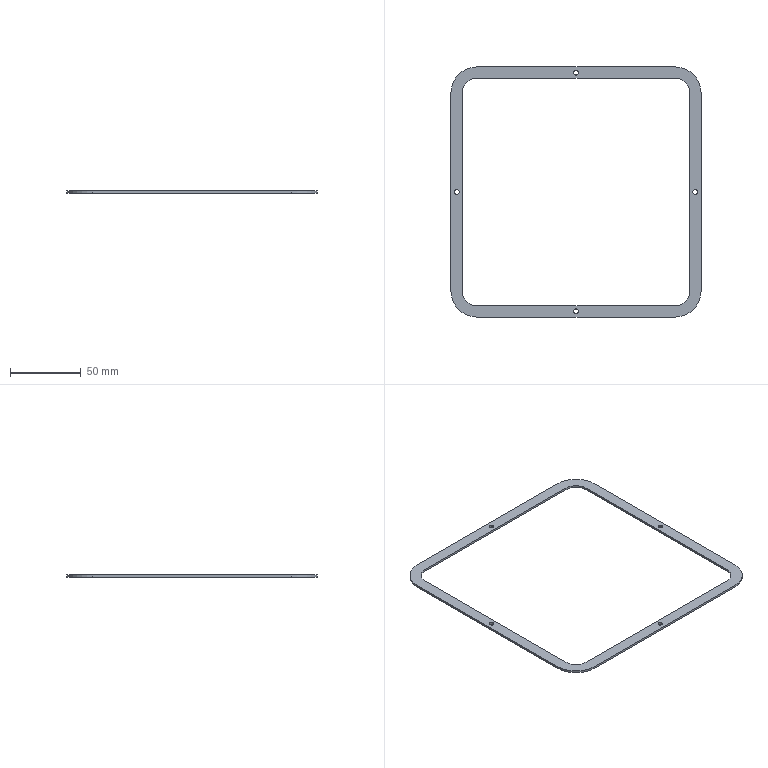Part | NX | features BREP 1 | 1 solid | 26 faces | box 176.2 x 176.2 x 1.5 mm | volume 7641 mm3 | cylinder 16 | plane 10 | commonest cylinder face diameters 3.2 x8 20.4 x4 36.2 x4
STEP:
#1=CARTESIAN_POINT('',(99.822,29.098,1.5));
#2=VERTEX_POINT('',#1);
#3=CARTESIAN_POINT('',(103.022,29.098,1.5));
#4=VERTEX_POINT('',#3);
#5=CARTESIAN_POINT('',(101.422,29.098,1.5));
#6=DIRECTION('',(0.,0.,1.));
#7=DIRECTION('',(1.,0.,0.));
#8=AXIS2_PLACEMENT_3D('',#5,#6,#7);
#9=CIRCLE('',#8,1.6);
#10=EDGE_CURVE('',#2,#4,#9,.T.);
#11=ORIENTED_EDGE('',*,*,#10,.T.);
#12=CARTESIAN_POINT('',(103.022,29.098,0.));
#13=VERTEX_POINT('',#12);
#14=CARTESIAN_POINT('',(103.022,29.098,1.5));
#15=DIRECTION('',(0.,0.,-1.));
#16=VECTOR('',#15,1000.);
#17=LINE('',#14,#16);
#18=EDGE_CURVE('',#13,#4,#17,.F.);
#19=ORIENTED_EDGE('',*,*,#18,.F.);
#20=CARTESIAN_POINT('',(99.822,29.098,0.));
#21=VERTEX_POINT('',#20);
#22=CARTESIAN_POINT('',(101.422,29.098,0.));
#23=DIRECTION('',(0.,0.,1.));
#24=DIRECTION('',(1.,0.,0.));
#25=AXIS2_PLACEMENT_3D('',#22,#23,#24);
#26=CIRCLE('',#25,1.6);
#27=EDGE_CURVE('',#21,#13,#26,.T.);
#28=ORIENTED_EDGE('',*,*,#27,.F.);
#29=CARTESIAN_POINT('',(99.822,29.098,1.5));
#30=DIRECTION('',(0.,0.,-1.));
#31=VECTOR('',#30,1000.);
#32=LINE('',#29,#31);
#33=EDGE_CURVE('',#21,#2,#32,.F.);
#34=ORIENTED_EDGE('',*,*,#33,.T.);
#35=EDGE_LOOP('',(#11,#19,#28,#34));
#36=FACE_BOUND('',#35,.T.);
#37=CARTESIAN_POINT('',(101.422,29.098,1.5));
#38=DIRECTION('',(0.,0.,-1.));
#39=DIRECTION('',(1.,0.,0.));
#40=AXIS2_PLACEMENT_3D('',#37,#38,#39);
#41=CYLINDRICAL_SURFACE('',#40,1.6);
#42=ADVANCED_FACE('',(#36),#41,.F.);
#43=CARTESIAN_POINT('',(15.822,-54.902,1.5));
#44=VERTEX_POINT('',#43);
#45=CARTESIAN_POINT('',(19.022,-54.902,1.5));
#46=VERTEX_POINT('',#45);
#47=CARTESIAN_POINT('',(17.422,-54.902,1.5));
#48=DIRECTION('',(0.,0.,1.));
#49=DIRECTION('',(1.,0.,0.));
#50=AXIS2_PLACEMENT_3D('',#47,#48,#49);
#51=CIRCLE('',#50,1.6);
#52=EDGE_CURVE('',#44,#46,#51,.T.);
#53=ORIENTED_EDGE('',*,*,#52,.T.);
#54=CARTESIAN_POINT('',(19.022,-54.902,0.));
#55=VERTEX_POINT('',#54);
#56=CARTESIAN_POINT('',(19.022,-54.902,1.5));
#57=DIRECTION('',(0.,0.,-1.));
#58=VECTOR('',#57,1000.);
#59=LINE('',#56,#58);
#60=EDGE_CURVE('',#55,#46,#59,.F.);
#61=ORIENTED_EDGE('',*,*,#60,.F.);
#62=CARTESIAN_POINT('',(15.822,-54.902,0.));
#63=VERTEX_POINT('',#62);
#64=CARTESIAN_POINT('',(17.422,-54.902,0.));
#65=DIRECTION('',(0.,0.,1.));
#66=DIRECTION('',(1.,0.,0.));
#67=AXIS2_PLACEMENT_3D('',#64,#65,#66);
#68=CIRCLE('',#67,1.6);
#69=EDGE_CURVE('',#63,#55,#68,.T.);
#70=ORIENTED_EDGE('',*,*,#69,.F.);
#71=CARTESIAN_POINT('',(15.822,-54.902,1.5));
#72=DIRECTION('',(0.,0.,-1.));
#73=VECTOR('',#72,1000.);
#74=LINE('',#71,#73);
#75=EDGE_CURVE('',#63,#44,#74,.F.);
#76=ORIENTED_EDGE('',*,*,#75,.T.);
#77=EDGE_LOOP('',(#53,#61,#70,#76));
#78=FACE_BOUND('',#77,.T.);
#79=CARTESIAN_POINT('',(17.422,-54.902,1.5));
#80=DIRECTION('',(0.,0.,-1.));
#81=DIRECTION('',(1.,0.,0.));
#82=AXIS2_PLACEMENT_3D('',#79,#80,#81);
#83=CYLINDRICAL_SURFACE('',#82,1.6);
#84=ADVANCED_FACE('',(#78),#83,.F.);
#85=CARTESIAN_POINT('',(-68.178,29.098,1.5));
#86=VERTEX_POINT('',#85);
#87=CARTESIAN_POINT('',(-64.978,29.098,1.5));
#88=VERTEX_POINT('',#87);
#89=CARTESIAN_POINT('',(-66.578,29.098,1.5));
#90=DIRECTION('',(0.,0.,1.));
#91=DIRECTION('',(1.,0.,0.));
#92=AXIS2_PLACEMENT_3D('',#89,#90,#91);
#93=CIRCLE('',#92,1.6);
#94=EDGE_CURVE('',#86,#88,#93,.T.);
#95=ORIENTED_EDGE('',*,*,#94,.T.);
#96=CARTESIAN_POINT('',(-64.978,29.098,0.));
#97=VERTEX_POINT('',#96);
#98=CARTESIAN_POINT('',(-64.978,29.098,1.5));
#99=DIRECTION('',(0.,0.,-1.));
#100=VECTOR('',#99,1000.);
#101=LINE('',#98,#100);
#102=EDGE_CURVE('',#97,#88,#101,.F.);
#103=ORIENTED_EDGE('',*,*,#102,.F.);
#104=CARTESIAN_POINT('',(-68.178,29.098,0.));
#105=VERTEX_POINT('',#104);
#106=CARTESIAN_POINT('',(-66.578,29.098,0.));
#107=DIRECTION('',(0.,0.,1.));
#108=DIRECTION('',(1.,0.,0.));
#109=AXIS2_PLACEMENT_3D('',#106,#107,#108);
#110=CIRCLE('',#109,1.6);
#111=EDGE_CURVE('',#105,#97,#110,.T.);
#112=ORIENTED_EDGE('',*,*,#111,.F.);
#113=CARTESIAN_POINT('',(-68.178,29.098,1.5));
#114=DIRECTION('',(0.,0.,-1.));
#115=VECTOR('',#114,1000.);
#116=LINE('',#113,#115);
#117=EDGE_CURVE('',#105,#86,#116,.F.);
#118=ORIENTED_EDGE('',*,*,#117,.T.);
#119=EDGE_LOOP('',(#95,#103,#112,#118));
#120=FACE_BOUND('',#119,.T.);
#121=CARTESIAN_POINT('',(-66.578,29.098,1.5));
#122=DIRECTION('',(0.,0.,-1.));
#123=DIRECTION('',(1.,0.,0.));
#124=AXIS2_PLACEMENT_3D('',#121,#122,#123);
#125=CYLINDRICAL_SURFACE('',#124,1.6);
#126=ADVANCED_FACE('',(#120),#125,.F.);
#127=CARTESIAN_POINT('',(15.822,113.098,1.5));
#128=VERTEX_POINT('',#127);
#129=CARTESIAN_POINT('',(19.022,113.098,1.5));
#130=VERTEX_POINT('',#129);
#131=CARTESIAN_POINT('',(17.422,113.098,1.5));
#132=DIRECTION('',(0.,0.,1.));
#133=DIRECTION('',(1.,0.,0.));
#134=AXIS2_PLACEMENT_3D('',#131,#132,#133);
#135=CIRCLE('',#134,1.6);
#136=EDGE_CURVE('',#128,#130,#135,.T.);
#137=ORIENTED_EDGE('',*,*,#136,.T.);
#138=CARTESIAN_POINT('',(19.022,113.098,0.));
#139=VERTEX_POINT('',#138);
#140=CARTESIAN_POINT('',(19.022,113.098,1.5));
#141=DIRECTION('',(0.,0.,-1.));
#142=VECTOR('',#141,1000.);
#143=LINE('',#140,#142);
#144=EDGE_CURVE('',#139,#130,#143,.F.);
#145=ORIENTED_EDGE('',*,*,#144,.F.);
#146=CARTESIAN_POINT('',(15.822,113.098,0.));
#147=VERTEX_POINT('',#146);
#148=CARTESIAN_POINT('',(17.422,113.098,0.));
#149=DIRECTION('',(0.,0.,1.));
#150=DIRECTION('',(1.,0.,0.));
#151=AXIS2_PLACEMENT_3D('',#148,#149,#150);
#152=CIRCLE('',#151,1.6);
#153=EDGE_CURVE('',#147,#139,#152,.T.);
#154=ORIENTED_EDGE('',*,*,#153,.F.);
#155=CARTESIAN_POINT('',(15.822,113.098,1.5));
#156=DIRECTION('',(0.,0.,-1.));
#157=VECTOR('',#156,1000.);
#158=LINE('',#155,#157);
#159=EDGE_CURVE('',#147,#128,#158,.F.);
#160=ORIENTED_EDGE('',*,*,#159,.T.);
#161=EDGE_LOOP('',(#137,#145,#154,#160));
#162=FACE_BOUND('',#161,.T.);
#163=CARTESIAN_POINT('',(17.422,113.098,1.5));
#164=DIRECTION('',(0.,0.,-1.));
#165=DIRECTION('',(1.,0.,0.));
#166=AXIS2_PLACEMENT_3D('',#163,#164,#165);
#167=CYLINDRICAL_SURFACE('',#166,1.6);
#168=ADVANCED_FACE('',(#162),#167,.F.);
#169=CARTESIAN_POINT('',(-70.678,-40.902,1.5));
#170=VERTEX_POINT('',#169);
#171=CARTESIAN_POINT('',(-52.578,-59.002,1.5));
#172=VERTEX_POINT('',#171);
#173=CARTESIAN_POINT('',(-52.578,-40.902,1.5));
#174=DIRECTION('',(0.,0.,1.));
#175=DIRECTION('',(1.,0.,0.));
#176=AXIS2_PLACEMENT_3D('',#173,#174,#175);
#177=CIRCLE('',#176,18.1);
#178=EDGE_CURVE('',#170,#172,#177,.T.);
#179=ORIENTED_EDGE('',*,*,#178,.T.);
#180=CARTESIAN_POINT('',(87.422,-59.002,1.5));
#181=VERTEX_POINT('',#180);
#182=CARTESIAN_POINT('',(-52.578,-59.002,1.5));
#183=DIRECTION('',(1.,0.,0.));
#184=VECTOR('',#183,1000.);
#185=LINE('',#182,#184);
#186=EDGE_CURVE('',#172,#181,#185,.T.);
#187=ORIENTED_EDGE('',*,*,#186,.T.);
#188=CARTESIAN_POINT('',(105.522,-40.902,1.5));
#189=VERTEX_POINT('',#188);
#190=CARTESIAN_POINT('',(87.422,-40.902,1.5));
#191=DIRECTION('',(0.,0.,1.));
#192=DIRECTION('',(1.,0.,0.));
#193=AXIS2_PLACEMENT_3D('',#190,#191,#192);
#194=CIRCLE('',#193,18.1);
#195=EDGE_CURVE('',#181,#189,#194,.T.);
#196=ORIENTED_EDGE('',*,*,#195,.T.);
#197=CARTESIAN_POINT('',(105.522,99.098,1.5));
#198=VERTEX_POINT('',#197);
#199=CARTESIAN_POINT('',(105.522,-40.902,1.5));
#200=DIRECTION('',(0.,1.,0.));
#201=VECTOR('',#200,1000.);
#202=LINE('',#199,#201);
#203=EDGE_CURVE('',#189,#198,#202,.T.);
#204=ORIENTED_EDGE('',*,*,#203,.T.);
#205=CARTESIAN_POINT('',(87.422,117.198,1.5));
#206=VERTEX_POINT('',#205);
#207=CARTESIAN_POINT('',(87.422,99.098,1.5));
#208=DIRECTION('',(0.,0.,1.));
#209=DIRECTION('',(1.,0.,0.));
#210=AXIS2_PLACEMENT_3D('',#207,#208,#209);
#211=CIRCLE('',#210,18.1);
#212=EDGE_CURVE('',#198,#206,#211,.T.);
#213=ORIENTED_EDGE('',*,*,#212,.T.);
#214=CARTESIAN_POINT('',(-52.578,117.198,1.5));
#215=VERTEX_POINT('',#214);
#216=CARTESIAN_POINT('',(87.422,117.198,1.5));
#217=DIRECTION('',(-1.,0.,0.));
#218=VECTOR('',#217,1000.);
#219=LINE('',#216,#218);
#220=EDGE_CURVE('',#206,#215,#219,.T.);
#221=ORIENTED_EDGE('',*,*,#220,.T.);
#222=CARTESIAN_POINT('',(-70.678,99.098,1.5));
#223=VERTEX_POINT('',#222);
#224=CARTESIAN_POINT('',(-52.578,99.098,1.5));
#225=DIRECTION('',(0.,0.,1.));
#226=DIRECTION('',(1.,0.,0.));
#227=AXIS2_PLACEMENT_3D('',#224,#225,#226);
#228=CIRCLE('',#227,18.1);
#229=EDGE_CURVE('',#215,#223,#228,.T.);
#230=ORIENTED_EDGE('',*,*,#229,.T.);
#231=CARTESIAN_POINT('',(-70.678,99.098,1.5));
#232=DIRECTION('',(0.,-1.,0.));
#233=VECTOR('',#232,1000.);
#234=LINE('',#231,#233);
#235=EDGE_CURVE('',#223,#170,#234,.T.);
#236=ORIENTED_EDGE('',*,*,#235,.T.);
#237=EDGE_LOOP('',(#179,#187,#196,#204,#213,#221,#230,#236));
#238=FACE_BOUND('',#237,.T.);
#239=ORIENTED_EDGE('',*,*,#52,.F.);
#240=CARTESIAN_POINT('',(17.422,-54.902,1.5));
#241=DIRECTION('',(0.,0.,1.));
#242=DIRECTION('',(1.,0.,0.));
#243=AXIS2_PLACEMENT_3D('',#240,#241,#242);
#244=CIRCLE('',#243,1.6);
#245=EDGE_CURVE('',#46,#44,#244,.T.);
#246=ORIENTED_EDGE('',*,*,#245,.F.);
#247=EDGE_LOOP('',(#239,#246));
#248=FACE_BOUND('',#247,.T.);
#249=ORIENTED_EDGE('',*,*,#136,.F.);
#250=CARTESIAN_POINT('',(17.422,113.098,1.5));
#251=DIRECTION('',(0.,0.,1.));
#252=DIRECTION('',(1.,0.,0.));
#253=AXIS2_PLACEMENT_3D('',#250,#251,#252);
#254=CIRCLE('',#253,1.6);
#255=EDGE_CURVE('',#130,#128,#254,.T.);
#256=ORIENTED_EDGE('',*,*,#255,.F.);
#257=EDGE_LOOP('',(#249,#256));
#258=FACE_BOUND('',#257,.T.);
#259=CARTESIAN_POINT('',(-52.578,-51.102,1.5));
#260=VERTEX_POINT('',#259);
#261=CARTESIAN_POINT('',(87.422,-51.102,1.5));
#262=VERTEX_POINT('',#261);
#263=CARTESIAN_POINT('',(-52.578,-51.102,1.5));
#264=DIRECTION('',(1.,0.,0.));
#265=VECTOR('',#264,1000.);
#266=LINE('',#263,#265);
#267=EDGE_CURVE('',#260,#262,#266,.T.);
#268=ORIENTED_EDGE('',*,*,#267,.F.);
#269=CARTESIAN_POINT('',(-62.778,-40.902,1.5));
#270=VERTEX_POINT('',#269);
#271=CARTESIAN_POINT('',(-52.578,-40.902,1.5));
#272=DIRECTION('',(0.,0.,1.));
#273=DIRECTION('',(1.,0.,0.));
#274=AXIS2_PLACEMENT_3D('',#271,#272,#273);
#275=CIRCLE('',#274,10.2);
#276=EDGE_CURVE('',#270,#260,#275,.T.);
#277=ORIENTED_EDGE('',*,*,#276,.F.);
#278=CARTESIAN_POINT('',(-62.778,99.098,1.5));
#279=VERTEX_POINT('',#278);
#280=CARTESIAN_POINT('',(-62.778,99.098,1.5));
#281=DIRECTION('',(0.,-1.,0.));
#282=VECTOR('',#281,1000.);
#283=LINE('',#280,#282);
#284=EDGE_CURVE('',#279,#270,#283,.T.);
#285=ORIENTED_EDGE('',*,*,#284,.F.);
#286=CARTESIAN_POINT('',(-52.578,109.298,1.5));
#287=VERTEX_POINT('',#286);
#288=CARTESIAN_POINT('',(-52.578,99.098,1.5));
#289=DIRECTION('',(0.,0.,1.));
#290=DIRECTION('',(1.,0.,0.));
#291=AXIS2_PLACEMENT_3D('',#288,#289,#290);
#292=CIRCLE('',#291,10.2);
#293=EDGE_CURVE('',#287,#279,#292,.T.);
#294=ORIENTED_EDGE('',*,*,#293,.F.);
#295=CARTESIAN_POINT('',(87.422,109.298,1.5));
#296=VERTEX_POINT('',#295);
#297=CARTESIAN_POINT('',(87.422,109.298,1.5));
#298=DIRECTION('',(-1.,0.,0.));
#299=VECTOR('',#298,1000.);
#300=LINE('',#297,#299);
#301=EDGE_CURVE('',#296,#287,#300,.T.);
#302=ORIENTED_EDGE('',*,*,#301,.F.);
#303=CARTESIAN_POINT('',(97.622,99.098,1.5));
#304=VERTEX_POINT('',#303);
#305=CARTESIAN_POINT('',(87.422,99.098,1.5));
#306=DIRECTION('',(0.,0.,1.));
#307=DIRECTION('',(1.,0.,0.));
#308=AXIS2_PLACEMENT_3D('',#305,#306,#307);
#309=CIRCLE('',#308,10.2);
#310=EDGE_CURVE('',#304,#296,#309,.T.);
#311=ORIENTED_EDGE('',*,*,#310,.F.);
#312=CARTESIAN_POINT('',(97.622,-40.902,1.5));
#313=VERTEX_POINT('',#312);
#314=CARTESIAN_POINT('',(97.622,-40.902,1.5));
#315=DIRECTION('',(0.,1.,0.));
#316=VECTOR('',#315,1000.);
#317=LINE('',#314,#316);
#318=EDGE_CURVE('',#313,#304,#317,.T.);
#319=ORIENTED_EDGE('',*,*,#318,.F.);
#320=CARTESIAN_POINT('',(87.422,-40.902,1.5));
#321=DIRECTION('',(0.,0.,1.));
#322=DIRECTION('',(1.,0.,0.));
#323=AXIS2_PLACEMENT_3D('',#320,#321,#322);
#324=CIRCLE('',#323,10.2);
#325=EDGE_CURVE('',#262,#313,#324,.T.);
#326=ORIENTED_EDGE('',*,*,#325,.F.);
#327=EDGE_LOOP('',(#268,#277,#285,#294,#302,#311,#319,#326));
#328=FACE_BOUND('',#327,.T.);
#329=ORIENTED_EDGE('',*,*,#94,.F.);
#330=CARTESIAN_POINT('',(-66.578,29.098,1.5));
#331=DIRECTION('',(0.,0.,1.));
#332=DIRECTION('',(1.,0.,0.));
#333=AXIS2_PLACEMENT_3D('',#330,#331,#332);
#334=CIRCLE('',#333,1.6);
#335=EDGE_CURVE('',#88,#86,#334,.T.);
#336=ORIENTED_EDGE('',*,*,#335,.F.);
#337=EDGE_LOOP('',(#329,#336));
#338=FACE_BOUND('',#337,.T.);
#339=ORIENTED_EDGE('',*,*,#10,.F.);
#340=CARTESIAN_POINT('',(101.422,29.098,1.5));
#341=DIRECTION('',(0.,0.,1.));
#342=DIRECTION('',(1.,0.,0.));
#343=AXIS2_PLACEMENT_3D('',#340,#341,#342);
#344=CIRCLE('',#343,1.6);
#345=EDGE_CURVE('',#4,#2,#344,.T.);
#346=ORIENTED_EDGE('',*,*,#345,.F.);
#347=EDGE_LOOP('',(#339,#346));
#348=FACE_BOUND('',#347,.T.);
#349=CARTESIAN_POINT('',(-52.578,-40.902,1.5));
#350=DIRECTION('',(0.,0.,1.));
#351=DIRECTION('',(-1.,0.,0.));
#352=AXIS2_PLACEMENT_3D('',#349,#350,#351);
#353=PLANE('',#352);
#354=ADVANCED_FACE('',(#238,#248,#258,#328,#338,#348),#353,.T.);
#355=CARTESIAN_POINT('',(-70.678,-40.902,0.));
#356=VERTEX_POINT('',#355);
#357=CARTESIAN_POINT('',(-52.578,-59.002,0.));
#358=VERTEX_POINT('',#357);
#359=CARTESIAN_POINT('',(-52.578,-40.902,0.));
#360=DIRECTION('',(0.,0.,1.));
#361=DIRECTION('',(1.,0.,0.));
#362=AXIS2_PLACEMENT_3D('',#359,#360,#361);
#363=CIRCLE('',#362,18.1);
#364=EDGE_CURVE('',#356,#358,#363,.T.);
#365=ORIENTED_EDGE('',*,*,#364,.F.);
#366=CARTESIAN_POINT('',(-70.678,99.098,0.));
#367=VERTEX_POINT('',#366);
#368=CARTESIAN_POINT('',(-70.678,99.098,0.));
#369=DIRECTION('',(0.,-1.,0.));
#370=VECTOR('',#369,1000.);
#371=LINE('',#368,#370);
#372=EDGE_CURVE('',#367,#356,#371,.T.);
#373=ORIENTED_EDGE('',*,*,#372,.F.);
#374=CARTESIAN_POINT('',(-52.578,117.198,0.));
#375=VERTEX_POINT('',#374);
#376=CARTESIAN_POINT('',(-52.578,99.098,0.));
#377=DIRECTION('',(0.,0.,1.));
#378=DIRECTION('',(1.,0.,0.));
#379=AXIS2_PLACEMENT_3D('',#376,#377,#378);
#380=CIRCLE('',#379,18.1);
#381=EDGE_CURVE('',#375,#367,#380,.T.);
#382=ORIENTED_EDGE('',*,*,#381,.F.);
#383=CARTESIAN_POINT('',(87.422,117.198,0.));
#384=VERTEX_POINT('',#383);
#385=CARTESIAN_POINT('',(87.422,117.198,0.));
#386=DIRECTION('',(-1.,0.,0.));
#387=VECTOR('',#386,1000.);
#388=LINE('',#385,#387);
#389=EDGE_CURVE('',#384,#375,#388,.T.);
#390=ORIENTED_EDGE('',*,*,#389,.F.);
#391=CARTESIAN_POINT('',(105.522,99.098,0.));
#392=VERTEX_POINT('',#391);
#393=CARTESIAN_POINT('',(87.422,99.098,0.));
#394=DIRECTION('',(0.,0.,1.));
#395=DIRECTION('',(1.,0.,0.));
#396=AXIS2_PLACEMENT_3D('',#393,#394,#395);
#397=CIRCLE('',#396,18.1);
#398=EDGE_CURVE('',#392,#384,#397,.T.);
#399=ORIENTED_EDGE('',*,*,#398,.F.);
#400=CARTESIAN_POINT('',(105.522,-40.902,0.));
#401=VERTEX_POINT('',#400);
#402=CARTESIAN_POINT('',(105.522,-40.902,0.));
#403=DIRECTION('',(0.,1.,0.));
#404=VECTOR('',#403,1000.);
#405=LINE('',#402,#404);
#406=EDGE_CURVE('',#401,#392,#405,.T.);
#407=ORIENTED_EDGE('',*,*,#406,.F.);
#408=CARTESIAN_POINT('',(87.422,-59.002,0.));
#409=VERTEX_POINT('',#408);
#410=CARTESIAN_POINT('',(87.422,-40.902,0.));
#411=DIRECTION('',(0.,0.,1.));
#412=DIRECTION('',(1.,0.,0.));
#413=AXIS2_PLACEMENT_3D('',#410,#411,#412);
#414=CIRCLE('',#413,18.1);
#415=EDGE_CURVE('',#409,#401,#414,.T.);
#416=ORIENTED_EDGE('',*,*,#415,.F.);
#417=CARTESIAN_POINT('',(-52.578,-59.002,0.));
#418=DIRECTION('',(1.,0.,0.));
#419=VECTOR('',#418,1000.);
#420=LINE('',#417,#419);
#421=EDGE_CURVE('',#358,#409,#420,.T.);
#422=ORIENTED_EDGE('',*,*,#421,.F.);
#423=EDGE_LOOP('',(#365,#373,#382,#390,#399,#407,#416,#422));
#424=FACE_BOUND('',#423,.T.);
#425=CARTESIAN_POINT('',(-62.778,-40.902,0.));
#426=VERTEX_POINT('',#425);
#427=CARTESIAN_POINT('',(-52.578,-51.102,0.));
#428=VERTEX_POINT('',#427);
#429=CARTESIAN_POINT('',(-52.578,-40.902,0.));
#430=DIRECTION('',(0.,0.,1.));
#431=DIRECTION('',(1.,0.,0.));
#432=AXIS2_PLACEMENT_3D('',#429,#430,#431);
#433=CIRCLE('',#432,10.2);
#434=EDGE_CURVE('',#426,#428,#433,.T.);
#435=ORIENTED_EDGE('',*,*,#434,.T.);
#436=CARTESIAN_POINT('',(87.422,-51.102,0.));
#437=VERTEX_POINT('',#436);
#438=CARTESIAN_POINT('',(-52.578,-51.102,0.));
#439=DIRECTION('',(1.,0.,0.));
#440=VECTOR('',#439,1000.);
#441=LINE('',#438,#440);
#442=EDGE_CURVE('',#428,#437,#441,.T.);
#443=ORIENTED_EDGE('',*,*,#442,.T.);
#444=CARTESIAN_POINT('',(97.622,-40.902,0.));
#445=VERTEX_POINT('',#444);
#446=CARTESIAN_POINT('',(87.422,-40.902,0.));
#447=DIRECTION('',(0.,0.,1.));
#448=DIRECTION('',(1.,0.,0.));
#449=AXIS2_PLACEMENT_3D('',#446,#447,#448);
#450=CIRCLE('',#449,10.2);
#451=EDGE_CURVE('',#437,#445,#450,.T.);
#452=ORIENTED_EDGE('',*,*,#451,.T.);
#453=CARTESIAN_POINT('',(97.622,99.098,0.));
#454=VERTEX_POINT('',#453);
#455=CARTESIAN_POINT('',(97.622,-40.902,0.));
#456=DIRECTION('',(0.,1.,0.));
#457=VECTOR('',#456,1000.);
#458=LINE('',#455,#457);
#459=EDGE_CURVE('',#445,#454,#458,.T.);
#460=ORIENTED_EDGE('',*,*,#459,.T.);
#461=CARTESIAN_POINT('',(87.422,109.298,0.));
#462=VERTEX_POINT('',#461);
#463=CARTESIAN_POINT('',(87.422,99.098,0.));
#464=DIRECTION('',(0.,0.,1.));
#465=DIRECTION('',(1.,0.,0.));
#466=AXIS2_PLACEMENT_3D('',#463,#464,#465);
#467=CIRCLE('',#466,10.2);
#468=EDGE_CURVE('',#454,#462,#467,.T.);
#469=ORIENTED_EDGE('',*,*,#468,.T.);
#470=CARTESIAN_POINT('',(-52.578,109.298,0.));
#471=VERTEX_POINT('',#470);
#472=CARTESIAN_POINT('',(87.422,109.298,0.));
#473=DIRECTION('',(-1.,0.,0.));
#474=VECTOR('',#473,1000.);
#475=LINE('',#472,#474);
#476=EDGE_CURVE('',#462,#471,#475,.T.);
#477=ORIENTED_EDGE('',*,*,#476,.T.);
#478=CARTESIAN_POINT('',(-62.778,99.098,0.));
#479=VERTEX_POINT('',#478);
#480=CARTESIAN_POINT('',(-52.578,99.098,0.));
#481=DIRECTION('',(0.,0.,1.));
#482=DIRECTION('',(1.,0.,0.));
#483=AXIS2_PLACEMENT_3D('',#480,#481,#482);
#484=CIRCLE('',#483,10.2);
#485=EDGE_CURVE('',#471,#479,#484,.T.);
#486=ORIENTED_EDGE('',*,*,#485,.T.);
#487=CARTESIAN_POINT('',(-62.778,99.098,0.));
#488=DIRECTION('',(0.,-1.,0.));
#489=VECTOR('',#488,1000.);
#490=LINE('',#487,#489);
#491=EDGE_CURVE('',#479,#426,#490,.T.);
#492=ORIENTED_EDGE('',*,*,#491,.T.);
#493=EDGE_LOOP('',(#435,#443,#452,#460,#469,#477,#486,#492));
#494=FACE_BOUND('',#493,.T.);
#495=ORIENTED_EDGE('',*,*,#153,.T.);
#496=CARTESIAN_POINT('',(17.422,113.098,0.));
#497=DIRECTION('',(0.,0.,1.));
#498=DIRECTION('',(1.,0.,0.));
#499=AXIS2_PLACEMENT_3D('',#496,#497,#498);
#500=CIRCLE('',#499,1.6);
#501=EDGE_CURVE('',#139,#147,#500,.T.);
#502=ORIENTED_EDGE('',*,*,#501,.T.);
#503=EDGE_LOOP('',(#495,#502));
#504=FACE_BOUND('',#503,.T.);
#505=ORIENTED_EDGE('',*,*,#111,.T.);
#506=CARTESIAN_POINT('',(-66.578,29.098,0.));
#507=DIRECTION('',(0.,0.,1.));
#508=DIRECTION('',(1.,0.,0.));
#509=AXIS2_PLACEMENT_3D('',#506,#507,#508);
#510=CIRCLE('',#509,1.6);
#511=EDGE_CURVE('',#97,#105,#510,.T.);
#512=ORIENTED_EDGE('',*,*,#511,.T.);
#513=EDGE_LOOP('',(#505,#512));
#514=FACE_BOUND('',#513,.T.);
#515=ORIENTED_EDGE('',*,*,#69,.T.);
#516=CARTESIAN_POINT('',(17.422,-54.902,0.));
#517=DIRECTION('',(0.,0.,1.));
#518=DIRECTION('',(1.,0.,0.));
#519=AXIS2_PLACEMENT_3D('',#516,#517,#518);
#520=CIRCLE('',#519,1.6);
#521=EDGE_CURVE('',#55,#63,#520,.T.);
#522=ORIENTED_EDGE('',*,*,#521,.T.);
#523=EDGE_LOOP('',(#515,#522));
#524=FACE_BOUND('',#523,.T.);
#525=ORIENTED_EDGE('',*,*,#27,.T.);
#526=CARTESIAN_POINT('',(101.422,29.098,0.));
#527=DIRECTION('',(0.,0.,1.));
#528=DIRECTION('',(1.,0.,0.));
#529=AXIS2_PLACEMENT_3D('',#526,#527,#528);
#530=CIRCLE('',#529,1.6);
#531=EDGE_CURVE('',#13,#21,#530,.T.);
#532=ORIENTED_EDGE('',*,*,#531,.T.);
#533=EDGE_LOOP('',(#525,#532));
#534=FACE_BOUND('',#533,.T.);
#535=CARTESIAN_POINT('',(-52.578,-40.902,0.));
#536=DIRECTION('',(0.,0.,1.));
#537=DIRECTION('',(-1.,0.,0.));
#538=AXIS2_PLACEMENT_3D('',#535,#536,#537);
#539=PLANE('',#538);
#540=ADVANCED_FACE('',(#424,#494,#504,#514,#524,#534),#539,.F.);
#541=ORIENTED_EDGE('',*,*,#364,.T.);
#542=CARTESIAN_POINT('',(-52.578,-59.002,1.5));
#543=DIRECTION('',(0.,0.,-1.));
#544=VECTOR('',#543,1000.);
#545=LINE('',#542,#544);
#546=EDGE_CURVE('',#172,#358,#545,.T.);
#547=ORIENTED_EDGE('',*,*,#546,.F.);
#548=ORIENTED_EDGE('',*,*,#178,.F.);
#549=CARTESIAN_POINT('',(-70.678,-40.902,1.5));
#550=DIRECTION('',(0.,0.,-1.));
#551=VECTOR('',#550,1000.);
#552=LINE('',#549,#551);
#553=EDGE_CURVE('',#170,#356,#552,.T.);
#554=ORIENTED_EDGE('',*,*,#553,.T.);
#555=EDGE_LOOP('',(#541,#547,#548,#554));
#556=FACE_BOUND('',#555,.T.);
#557=CARTESIAN_POINT('',(-52.578,-40.902,1.5));
#558=DIRECTION('',(0.,0.,-1.));
#559=DIRECTION('',(1.,0.,0.));
#560=AXIS2_PLACEMENT_3D('',#557,#558,#559);
#561=CYLINDRICAL_SURFACE('',#560,18.1);
#562=ADVANCED_FACE('',(#556),#561,.T.);
#563=ORIENTED_EDGE('',*,*,#421,.T.);
#564=CARTESIAN_POINT('',(87.422,-59.002,1.5));
#565=DIRECTION('',(0.,0.,-1.));
#566=VECTOR('',#565,1000.);
#567=LINE('',#564,#566);
#568=EDGE_CURVE('',#181,#409,#567,.T.);
#569=ORIENTED_EDGE('',*,*,#568,.F.);
#570=ORIENTED_EDGE('',*,*,#186,.F.);
#571=ORIENTED_EDGE('',*,*,#546,.T.);
#572=EDGE_LOOP('',(#563,#569,#570,#571));
#573=FACE_BOUND('',#572,.T.);
#574=CARTESIAN_POINT('',(-52.578,-59.002,1.5));
#575=DIRECTION('',(0.,1.,0.));
#576=DIRECTION('',(-1.,0.,0.));
#577=AXIS2_PLACEMENT_3D('',#574,#575,#576);
#578=PLANE('',#577);
#579=ADVANCED_FACE('',(#573),#578,.F.);
#580=ORIENTED_EDGE('',*,*,#415,.T.);
#581=CARTESIAN_POINT('',(105.522,-40.902,1.5));
#582=DIRECTION('',(0.,0.,-1.));
#583=VECTOR('',#582,1000.);
#584=LINE('',#581,#583);
#585=EDGE_CURVE('',#189,#401,#584,.T.);
#586=ORIENTED_EDGE('',*,*,#585,.F.);
#587=ORIENTED_EDGE('',*,*,#195,.F.);
#588=ORIENTED_EDGE('',*,*,#568,.T.);
#589=EDGE_LOOP('',(#580,#586,#587,#588));
#590=FACE_BOUND('',#589,.T.);
#591=CARTESIAN_POINT('',(87.422,-40.902,1.5));
#592=DIRECTION('',(0.,0.,-1.));
#593=DIRECTION('',(1.,0.,0.));
#594=AXIS2_PLACEMENT_3D('',#591,#592,#593);
#595=CYLINDRICAL_SURFACE('',#594,18.1);
#596=ADVANCED_FACE('',(#590),#595,.T.);
#597=ORIENTED_EDGE('',*,*,#406,.T.);
#598=CARTESIAN_POINT('',(105.522,99.098,1.5));
#599=DIRECTION('',(0.,0.,-1.));
#600=VECTOR('',#599,1000.);
#601=LINE('',#598,#600);
#602=EDGE_CURVE('',#198,#392,#601,.T.);
#603=ORIENTED_EDGE('',*,*,#602,.F.);
#604=ORIENTED_EDGE('',*,*,#203,.F.);
#605=ORIENTED_EDGE('',*,*,#585,.T.);
#606=EDGE_LOOP('',(#597,#603,#604,#605));
#607=FACE_BOUND('',#606,.T.);
#608=CARTESIAN_POINT('',(105.522,-40.902,1.5));
#609=DIRECTION('',(-1.,0.,0.));
#610=DIRECTION('',(0.,0.,-1.));
#611=AXIS2_PLACEMENT_3D('',#608,#609,#610);
#612=PLANE('',#611);
#613=ADVANCED_FACE('',(#607),#612,.F.);
#614=ORIENTED_EDGE('',*,*,#398,.T.);
#615=CARTESIAN_POINT('',(87.422,117.198,1.5));
#616=DIRECTION('',(0.,0.,-1.));
#617=VECTOR('',#616,1000.);
#618=LINE('',#615,#617);
#619=EDGE_CURVE('',#206,#384,#618,.T.);
#620=ORIENTED_EDGE('',*,*,#619,.F.);
#621=ORIENTED_EDGE('',*,*,#212,.F.);
#622=ORIENTED_EDGE('',*,*,#602,.T.);
#623=EDGE_LOOP('',(#614,#620,#621,#622));
#624=FACE_BOUND('',#623,.T.);
#625=CARTESIAN_POINT('',(87.422,99.098,1.5));
#626=DIRECTION('',(0.,0.,-1.));
#627=DIRECTION('',(1.,0.,0.));
#628=AXIS2_PLACEMENT_3D('',#625,#626,#627);
#629=CYLINDRICAL_SURFACE('',#628,18.1);
#630=ADVANCED_FACE('',(#624),#629,.T.);
#631=ORIENTED_EDGE('',*,*,#389,.T.);
#632=CARTESIAN_POINT('',(-52.578,117.198,1.5));
#633=DIRECTION('',(0.,0.,-1.));
#634=VECTOR('',#633,1000.);
#635=LINE('',#632,#634);
#636=EDGE_CURVE('',#215,#375,#635,.T.);
#637=ORIENTED_EDGE('',*,*,#636,.F.);
#638=ORIENTED_EDGE('',*,*,#220,.F.);
#639=ORIENTED_EDGE('',*,*,#619,.T.);
#640=EDGE_LOOP('',(#631,#637,#638,#639));
#641=FACE_BOUND('',#640,.T.);
#642=CARTESIAN_POINT('',(87.422,117.198,1.5));
#643=DIRECTION('',(0.,-1.,0.));
#644=DIRECTION('',(0.,0.,1.));
#645=AXIS2_PLACEMENT_3D('',#642,#643,#644);
#646=PLANE('',#645);
#647=ADVANCED_FACE('',(#641),#646,.F.);
#648=ORIENTED_EDGE('',*,*,#381,.T.);
#649=CARTESIAN_POINT('',(-70.678,99.098,1.5));
#650=DIRECTION('',(0.,0.,-1.));
#651=VECTOR('',#650,1000.);
#652=LINE('',#649,#651);
#653=EDGE_CURVE('',#223,#367,#652,.T.);
#654=ORIENTED_EDGE('',*,*,#653,.F.);
#655=ORIENTED_EDGE('',*,*,#229,.F.);
#656=ORIENTED_EDGE('',*,*,#636,.T.);
#657=EDGE_LOOP('',(#648,#654,#655,#656));
#658=FACE_BOUND('',#657,.T.);
#659=CARTESIAN_POINT('',(-52.578,99.098,1.5));
#660=DIRECTION('',(0.,0.,-1.));
#661=DIRECTION('',(1.,0.,0.));
#662=AXIS2_PLACEMENT_3D('',#659,#660,#661);
#663=CYLINDRICAL_SURFACE('',#662,18.1);
#664=ADVANCED_FACE('',(#658),#663,.T.);
#665=ORIENTED_EDGE('',*,*,#372,.T.);
#666=ORIENTED_EDGE('',*,*,#553,.F.);
#667=ORIENTED_EDGE('',*,*,#235,.F.);
#668=ORIENTED_EDGE('',*,*,#653,.T.);
#669=EDGE_LOOP('',(#665,#666,#667,#668));
#670=FACE_BOUND('',#669,.T.);
#671=CARTESIAN_POINT('',(-70.678,99.098,1.5));
#672=DIRECTION('',(1.,0.,0.));
#673=DIRECTION('',(0.,0.,-1.));
#674=AXIS2_PLACEMENT_3D('',#671,#672,#673);
#675=PLANE('',#674);
#676=ADVANCED_FACE('',(#670),#675,.F.);
#677=ORIENTED_EDGE('',*,*,#434,.F.);
#678=CARTESIAN_POINT('',(-62.778,-40.902,1.5));
#679=DIRECTION('',(0.,0.,-1.));
#680=VECTOR('',#679,1000.);
#681=LINE('',#678,#680);
#682=EDGE_CURVE('',#270,#426,#681,.T.);
#683=ORIENTED_EDGE('',*,*,#682,.F.);
#684=ORIENTED_EDGE('',*,*,#276,.T.);
#685=CARTESIAN_POINT('',(-52.578,-51.102,1.5));
#686=DIRECTION('',(0.,0.,-1.));
#687=VECTOR('',#686,1000.);
#688=LINE('',#685,#687);
#689=EDGE_CURVE('',#260,#428,#688,.T.);
#690=ORIENTED_EDGE('',*,*,#689,.T.);
#691=EDGE_LOOP('',(#677,#683,#684,#690));
#692=FACE_BOUND('',#691,.T.);
#693=CARTESIAN_POINT('',(-52.578,-40.902,1.5));
#694=DIRECTION('',(0.,0.,-1.));
#695=DIRECTION('',(1.,0.,0.));
#696=AXIS2_PLACEMENT_3D('',#693,#694,#695);
#697=CYLINDRICAL_SURFACE('',#696,10.2);
#698=ADVANCED_FACE('',(#692),#697,.F.);
#699=ORIENTED_EDGE('',*,*,#442,.F.);
#700=ORIENTED_EDGE('',*,*,#689,.F.);
#701=ORIENTED_EDGE('',*,*,#267,.T.);
#702=CARTESIAN_POINT('',(87.422,-51.102,1.5));
#703=DIRECTION('',(0.,0.,-1.));
#704=VECTOR('',#703,1000.);
#705=LINE('',#702,#704);
#706=EDGE_CURVE('',#262,#437,#705,.T.);
#707=ORIENTED_EDGE('',*,*,#706,.T.);
#708=EDGE_LOOP('',(#699,#700,#701,#707));
#709=FACE_BOUND('',#708,.T.);
#710=CARTESIAN_POINT('',(-52.578,-51.102,1.5));
#711=DIRECTION('',(0.,1.,0.));
#712=DIRECTION('',(-1.,0.,0.));
#713=AXIS2_PLACEMENT_3D('',#710,#711,#712);
#714=PLANE('',#713);
#715=ADVANCED_FACE('',(#709),#714,.T.);
#716=ORIENTED_EDGE('',*,*,#451,.F.);
#717=ORIENTED_EDGE('',*,*,#706,.F.);
#718=ORIENTED_EDGE('',*,*,#325,.T.);
#719=CARTESIAN_POINT('',(97.622,-40.902,1.5));
#720=DIRECTION('',(0.,0.,-1.));
#721=VECTOR('',#720,1000.);
#722=LINE('',#719,#721);
#723=EDGE_CURVE('',#313,#445,#722,.T.);
#724=ORIENTED_EDGE('',*,*,#723,.T.);
#725=EDGE_LOOP('',(#716,#717,#718,#724));
#726=FACE_BOUND('',#725,.T.);
#727=CARTESIAN_POINT('',(87.422,-40.902,1.5));
#728=DIRECTION('',(0.,0.,-1.));
#729=DIRECTION('',(1.,0.,0.));
#730=AXIS2_PLACEMENT_3D('',#727,#728,#729);
#731=CYLINDRICAL_SURFACE('',#730,10.2);
#732=ADVANCED_FACE('',(#726),#731,.F.);
#733=ORIENTED_EDGE('',*,*,#459,.F.);
#734=ORIENTED_EDGE('',*,*,#723,.F.);
#735=ORIENTED_EDGE('',*,*,#318,.T.);
#736=CARTESIAN_POINT('',(97.622,99.098,1.5));
#737=DIRECTION('',(0.,0.,-1.));
#738=VECTOR('',#737,1000.);
#739=LINE('',#736,#738);
#740=EDGE_CURVE('',#304,#454,#739,.T.);
#741=ORIENTED_EDGE('',*,*,#740,.T.);
#742=EDGE_LOOP('',(#733,#734,#735,#741));
#743=FACE_BOUND('',#742,.T.);
#744=CARTESIAN_POINT('',(97.622,-40.902,1.5));
#745=DIRECTION('',(-1.,0.,0.));
#746=DIRECTION('',(0.,-1.,0.));
#747=AXIS2_PLACEMENT_3D('',#744,#745,#746);
#748=PLANE('',#747);
#749=ADVANCED_FACE('',(#743),#748,.T.);
#750=ORIENTED_EDGE('',*,*,#468,.F.);
#751=ORIENTED_EDGE('',*,*,#740,.F.);
#752=ORIENTED_EDGE('',*,*,#310,.T.);
#753=CARTESIAN_POINT('',(87.422,109.298,1.5));
#754=DIRECTION('',(0.,0.,-1.));
#755=VECTOR('',#754,1000.);
#756=LINE('',#753,#755);
#757=EDGE_CURVE('',#296,#462,#756,.T.);
#758=ORIENTED_EDGE('',*,*,#757,.T.);
#759=EDGE_LOOP('',(#750,#751,#752,#758));
#760=FACE_BOUND('',#759,.T.);
#761=CARTESIAN_POINT('',(87.422,99.098,1.5));
#762=DIRECTION('',(0.,0.,-1.));
#763=DIRECTION('',(1.,0.,0.));
#764=AXIS2_PLACEMENT_3D('',#761,#762,#763);
#765=CYLINDRICAL_SURFACE('',#764,10.2);
#766=ADVANCED_FACE('',(#760),#765,.F.);
#767=ORIENTED_EDGE('',*,*,#476,.F.);
#768=ORIENTED_EDGE('',*,*,#757,.F.);
#769=ORIENTED_EDGE('',*,*,#301,.T.);
#770=CARTESIAN_POINT('',(-52.578,109.298,1.5));
#771=DIRECTION('',(0.,0.,-1.));
#772=VECTOR('',#771,1000.);
#773=LINE('',#770,#772);
#774=EDGE_CURVE('',#287,#471,#773,.T.);
#775=ORIENTED_EDGE('',*,*,#774,.T.);
#776=EDGE_LOOP('',(#767,#768,#769,#775));
#777=FACE_BOUND('',#776,.T.);
#778=CARTESIAN_POINT('',(87.422,109.298,1.5));
#779=DIRECTION('',(0.,-1.,0.));
#780=DIRECTION('',(0.,0.,1.));
#781=AXIS2_PLACEMENT_3D('',#778,#779,#780);
#782=PLANE('',#781);
#783=ADVANCED_FACE('',(#777),#782,.T.);
#784=ORIENTED_EDGE('',*,*,#485,.F.);
#785=ORIENTED_EDGE('',*,*,#774,.F.);
#786=ORIENTED_EDGE('',*,*,#293,.T.);
#787=CARTESIAN_POINT('',(-62.778,99.098,1.5));
#788=DIRECTION('',(0.,0.,-1.));
#789=VECTOR('',#788,1000.);
#790=LINE('',#787,#789);
#791=EDGE_CURVE('',#279,#479,#790,.T.);
#792=ORIENTED_EDGE('',*,*,#791,.T.);
#793=EDGE_LOOP('',(#784,#785,#786,#792));
#794=FACE_BOUND('',#793,.T.);
#795=CARTESIAN_POINT('',(-52.578,99.098,1.5));
#796=DIRECTION('',(0.,0.,-1.));
#797=DIRECTION('',(1.,0.,0.));
#798=AXIS2_PLACEMENT_3D('',#795,#796,#797);
#799=CYLINDRICAL_SURFACE('',#798,10.2);
#800=ADVANCED_FACE('',(#794),#799,.F.);
#801=ORIENTED_EDGE('',*,*,#491,.F.);
#802=ORIENTED_EDGE('',*,*,#791,.F.);
#803=ORIENTED_EDGE('',*,*,#284,.T.);
#804=ORIENTED_EDGE('',*,*,#682,.T.);
#805=EDGE_LOOP('',(#801,#802,#803,#804));
#806=FACE_BOUND('',#805,.T.);
#807=CARTESIAN_POINT('',(-62.778,99.098,1.5));
#808=DIRECTION('',(1.,0.,0.));
#809=DIRECTION('',(0.,0.,-1.));
#810=AXIS2_PLACEMENT_3D('',#807,#808,#809);
#811=PLANE('',#810);
#812=ADVANCED_FACE('',(#806),#811,.T.);
#813=ORIENTED_EDGE('',*,*,#144,.T.);
#814=ORIENTED_EDGE('',*,*,#255,.T.);
#815=ORIENTED_EDGE('',*,*,#159,.F.);
#816=ORIENTED_EDGE('',*,*,#501,.F.);
#817=EDGE_LOOP('',(#813,#814,#815,#816));
#818=FACE_BOUND('',#817,.T.);
#819=CARTESIAN_POINT('',(17.422,113.098,1.5));
#820=DIRECTION('',(0.,0.,-1.));
#821=DIRECTION('',(1.,0.,0.));
#822=AXIS2_PLACEMENT_3D('',#819,#820,#821);
#823=CYLINDRICAL_SURFACE('',#822,1.6);
#824=ADVANCED_FACE('',(#818),#823,.F.);
#825=ORIENTED_EDGE('',*,*,#102,.T.);
#826=ORIENTED_EDGE('',*,*,#335,.T.);
#827=ORIENTED_EDGE('',*,*,#117,.F.);
#828=ORIENTED_EDGE('',*,*,#511,.F.);
#829=EDGE_LOOP('',(#825,#826,#827,#828));
#830=FACE_BOUND('',#829,.T.);
#831=CARTESIAN_POINT('',(-66.578,29.098,1.5));
#832=DIRECTION('',(0.,0.,-1.));
#833=DIRECTION('',(1.,0.,0.));
#834=AXIS2_PLACEMENT_3D('',#831,#832,#833);
#835=CYLINDRICAL_SURFACE('',#834,1.6);
#836=ADVANCED_FACE('',(#830),#835,.F.);
#837=ORIENTED_EDGE('',*,*,#60,.T.);
#838=ORIENTED_EDGE('',*,*,#245,.T.);
#839=ORIENTED_EDGE('',*,*,#75,.F.);
#840=ORIENTED_EDGE('',*,*,#521,.F.);
#841=EDGE_LOOP('',(#837,#838,#839,#840));
#842=FACE_BOUND('',#841,.T.);
#843=CARTESIAN_POINT('',(17.422,-54.902,1.5));
#844=DIRECTION('',(0.,0.,-1.));
#845=DIRECTION('',(1.,0.,0.));
#846=AXIS2_PLACEMENT_3D('',#843,#844,#845);
#847=CYLINDRICAL_SURFACE('',#846,1.6);
#848=ADVANCED_FACE('',(#842),#847,.F.);
#849=ORIENTED_EDGE('',*,*,#18,.T.);
#850=ORIENTED_EDGE('',*,*,#345,.T.);
#851=ORIENTED_EDGE('',*,*,#33,.F.);
#852=ORIENTED_EDGE('',*,*,#531,.F.);
#853=EDGE_LOOP('',(#849,#850,#851,#852));
#854=FACE_BOUND('',#853,.T.);
#855=CARTESIAN_POINT('',(101.422,29.098,1.5));
#856=DIRECTION('',(0.,0.,-1.));
#857=DIRECTION('',(1.,0.,0.));
#858=AXIS2_PLACEMENT_3D('',#855,#856,#857);
#859=CYLINDRICAL_SURFACE('',#858,1.6);
#860=ADVANCED_FACE('',(#854),#859,.F.);
#861=CLOSED_SHELL('',(#42,#84,#126,#168,#354,#540,#562,#579,#596,#613,#630,#647,#664,#676,#698,#715,#732,#749,#766,#783,#800,#812,#824,#836,#848,#860));
#862=MANIFOLD_SOLID_BREP('',#861);
#863=(LENGTH_UNIT()NAMED_UNIT(*)SI_UNIT(.MILLI.,.METRE.));
#864=UNCERTAINTY_MEASURE_WITH_UNIT(LENGTH_MEASURE(0.00001),#863,'','');
#865=(NAMED_UNIT(*)PLANE_ANGLE_UNIT()SI_UNIT($,.RADIAN.));
#866=(NAMED_UNIT(*)SI_UNIT($,.STERADIAN.)SOLID_ANGLE_UNIT());
#867=(GEOMETRIC_REPRESENTATION_CONTEXT(3)GLOBAL_UNCERTAINTY_ASSIGNED_CONTEXT((#864))GLOBAL_UNIT_ASSIGNED_CONTEXT((#863,#865,#866))REPRESENTATION_CONTEXT('',''));
#868=ADVANCED_BREP_SHAPE_REPRESENTATION('',(#862),#867);